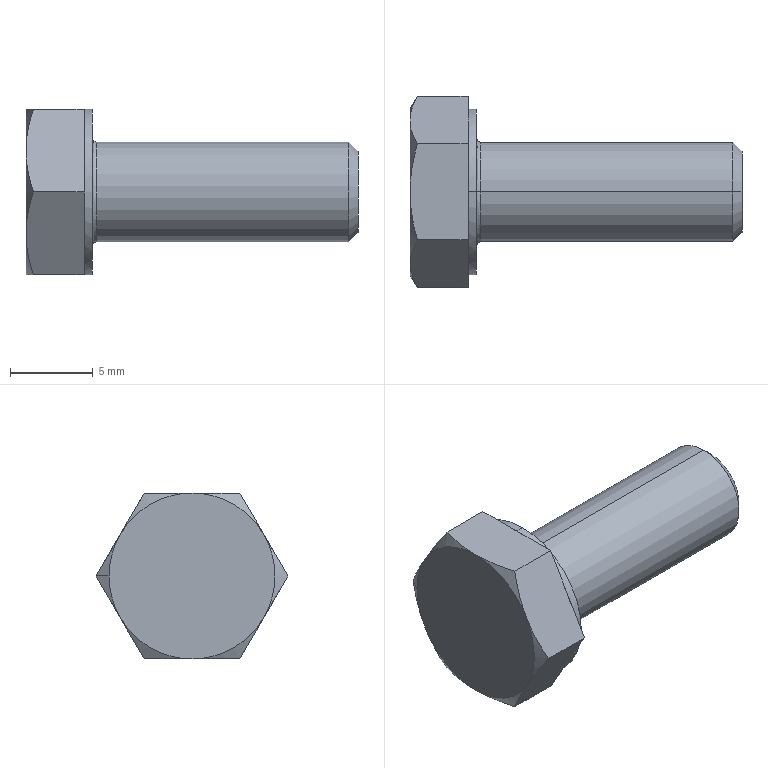Part | STEP file | Microwave Drying Flat Conveyor-hex screw gradeab_din_DIN EN 24017 - M6 x 16-N_Default | 1 solid | 30 faces | box 20 x 11.547 x 10 mm | volume 791.21 mm3 | plane 15 | cone 9 | cylinder 4 | spline 2 | commonest cylinder face diameters 6 x2 10 x2
STEP:
#1=CARTESIAN_POINT('',(4.,0.,3.25));
#2=VERTEX_POINT('',#1);
#3=CARTESIAN_POINT('',(4.,0.,-3.25));
#4=VERTEX_POINT('',#3);
#5=CARTESIAN_POINT('',(4.,0.,3.25));
#6=CARTESIAN_POINT('',(4.,0.2065,3.25));
#7=CARTESIAN_POINT('',(4.,0.511,3.221));
#8=CARTESIAN_POINT('',(4.,0.8568,3.138));
#9=CARTESIAN_POINT('',(4.,1.027,3.084));
#10=CARTESIAN_POINT('',(4.,1.1,3.058));
#11=CARTESIAN_POINT('',(4.,1.148,3.041));
#12=CARTESIAN_POINT('',(4.,1.17,3.032));
#13=CARTESIAN_POINT('',(4.,1.613,2.857));
#14=CARTESIAN_POINT('',(4.,1.981,2.615));
#15=CARTESIAN_POINT('',(4.,2.457,2.14));
#16=CARTESIAN_POINT('',(4.,2.666,1.883));
#17=CARTESIAN_POINT('',(4.,2.861,1.551));
#18=CARTESIAN_POINT('',(4.,2.945,1.376));
#19=CARTESIAN_POINT('',(4.,2.985,1.287));
#20=CARTESIAN_POINT('',(4.,3.001,1.248));
#21=CARTESIAN_POINT('',(4.,3.011,1.222));
#22=CARTESIAN_POINT('',(4.,3.017,1.208));
#23=CARTESIAN_POINT('',(4.,3.174,0.8124));
#24=CARTESIAN_POINT('',(4.,3.25,0.4129));
#25=CARTESIAN_POINT('',(4.,3.25,-0.2065));
#26=CARTESIAN_POINT('',(4.,3.222,-0.5109));
#27=CARTESIAN_POINT('',(4.,3.138,-0.8567));
#28=CARTESIAN_POINT('',(4.,3.084,-1.027));
#29=CARTESIAN_POINT('',(4.,3.058,-1.1));
#30=CARTESIAN_POINT('',(4.,3.041,-1.148));
#31=CARTESIAN_POINT('',(4.,3.032,-1.17));
#32=CARTESIAN_POINT('',(4.,2.857,-1.613));
#33=CARTESIAN_POINT('',(4.,2.615,-1.981));
#34=CARTESIAN_POINT('',(4.,2.14,-2.457));
#35=CARTESIAN_POINT('',(4.,1.883,-2.666));
#36=CARTESIAN_POINT('',(4.,1.551,-2.861));
#37=CARTESIAN_POINT('',(4.,1.376,-2.945));
#38=CARTESIAN_POINT('',(4.,1.3,-2.979));
#39=CARTESIAN_POINT('',(4.,1.248,-3.001));
#40=CARTESIAN_POINT('',(4.,1.22,-3.012));
#41=CARTESIAN_POINT('',(4.,0.8122,-3.174));
#42=CARTESIAN_POINT('',(4.,0.4135,-3.25));
#43=CARTESIAN_POINT('',(4.,0.,-3.25));
#44=B_SPLINE_CURVE_WITH_KNOTS('',3,(#5,#6,#7,#8,#9,#10,#11,#12,#13,#14,#15,#16,#17,#18,#19,#20,#21,#22,#23,#24,#25,#26,#27,#28,#29,#30,#31,#32,#33,#34,#35,#36,#37,#38,#39,#40,#41,#42,#43),.UNSPECIFIED.,.F.,.F.,(4,1,1,1,2,2,2,1,1,1,1,2,2,2,1,1,1,2,2,2,1,1,1,2,2,4),(0.,0.0625,0.09375,0.1094,0.1172,0.125,0.25,0.3125,0.3437,0.3594,0.3672,0.3711,0.375,0.5,0.5625,0.5937,0.6094,0.6172,0.625,0.75,0.8125,0.8437,0.8594,0.8672,0.875,1.),.UNSPECIFIED.);
#45=EDGE_CURVE('',#2,#4,#44,.T.);
#46=ORIENTED_EDGE('',*,*,#45,.F.);
#47=CARTESIAN_POINT('',(4.25,0.,3.));
#48=VERTEX_POINT('',#47);
#49=CARTESIAN_POINT('',(4.25,0.,3.25));
#50=DIRECTION('',(0.,-1.,0.));
#51=DIRECTION('',(0.,0.,1.));
#52=AXIS2_PLACEMENT_3D('',#49,#50,#51);
#53=CIRCLE('',#52,0.25);
#54=EDGE_CURVE('',#2,#48,#53,.T.);
#55=ORIENTED_EDGE('',*,*,#54,.T.);
#56=CARTESIAN_POINT('',(4.25,0.,-3.));
#57=VERTEX_POINT('',#56);
#58=CARTESIAN_POINT('',(4.25,0.,0.));
#59=DIRECTION('',(1.,0.,0.));
#60=DIRECTION('',(0.,0.,1.));
#61=AXIS2_PLACEMENT_3D('',#58,#59,#60);
#62=CIRCLE('',#61,3.);
#63=EDGE_CURVE('',#57,#48,#62,.T.);
#64=ORIENTED_EDGE('',*,*,#63,.F.);
#65=CARTESIAN_POINT('',(4.25,0.,-3.25));
#66=DIRECTION('',(0.,1.,0.));
#67=DIRECTION('',(0.,0.,-1.));
#68=AXIS2_PLACEMENT_3D('',#65,#66,#67);
#69=CIRCLE('',#68,0.25);
#70=EDGE_CURVE('',#4,#57,#69,.T.);
#71=ORIENTED_EDGE('',*,*,#70,.F.);
#72=EDGE_LOOP('',(#46,#55,#64,#71));
#73=FACE_OUTER_BOUND('',#72,.T.);
#74=CARTESIAN_POINT('',(4.,0.,-3.25));
#75=CARTESIAN_POINT('',(4.,6.5,-3.25));
#76=CARTESIAN_POINT('',(4.,6.5,3.25));
#77=CARTESIAN_POINT('',(4.,0.,3.25));
#78=CARTESIAN_POINT('',(4.,0.,-3.104));
#79=CARTESIAN_POINT('',(4.,6.207,-3.104));
#80=CARTESIAN_POINT('',(4.,6.207,3.104));
#81=CARTESIAN_POINT('',(4.,0.,3.104));
#82=CARTESIAN_POINT('',(4.104,0.,-3.));
#83=CARTESIAN_POINT('',(4.104,6.,-3.));
#84=CARTESIAN_POINT('',(4.104,6.,3.));
#85=CARTESIAN_POINT('',(4.104,0.,3.));
#86=CARTESIAN_POINT('',(4.25,0.,-3.));
#87=CARTESIAN_POINT('',(4.25,6.,-3.));
#88=CARTESIAN_POINT('',(4.25,6.,3.));
#89=CARTESIAN_POINT('',(4.25,0.,3.));
#90=(BOUNDED_SURFACE()B_SPLINE_SURFACE(3,3,((#74,#75,#76,#77),(#78,#79,#80,#81),(#82,#83,#84,#85),(#86,#87,#88,#89)),.UNSPECIFIED.,.F.,.F.,.T.)B_SPLINE_SURFACE_WITH_KNOTS((4,4),(4,4),(0.,1.),(0.,1.),.UNSPECIFIED.)GEOMETRIC_REPRESENTATION_ITEM()RATIONAL_B_SPLINE_SURFACE(((1.,0.3333,0.3333,1.),(0.8047,0.2682,0.2682,0.8047),(0.8047,0.2682,0.2682,0.8047),(1.,0.3333,0.3333,1.)))REPRESENTATION_ITEM('')SURFACE());
#91=ADVANCED_FACE('',(#73),#90,.F.);
#92=CARTESIAN_POINT('',(19.445,0.,3.));
#93=VERTEX_POINT('',#92);
#94=CARTESIAN_POINT('',(19.445,0.,-3.));
#95=VERTEX_POINT('',#94);
#96=CARTESIAN_POINT('',(19.445,0.,0.));
#97=DIRECTION('',(-1.,0.,0.));
#98=DIRECTION('',(0.,0.,1.));
#99=AXIS2_PLACEMENT_3D('',#96,#97,#98);
#100=CIRCLE('',#99,3.);
#101=EDGE_CURVE('',#93,#95,#100,.T.);
#102=ORIENTED_EDGE('',*,*,#101,.T.);
#103=CARTESIAN_POINT('',(0.,0.,-3.));
#104=DIRECTION('',(-1.,0.,0.));
#105=VECTOR('',#104,1000.);
#106=LINE('',#103,#105);
#107=EDGE_CURVE('',#95,#57,#106,.T.);
#108=ORIENTED_EDGE('',*,*,#107,.T.);
#109=ORIENTED_EDGE('',*,*,#63,.T.);
#110=CARTESIAN_POINT('',(0.,0.,3.));
#111=DIRECTION('',(-1.,0.,0.));
#112=VECTOR('',#111,1000.);
#113=LINE('',#110,#112);
#114=EDGE_CURVE('',#93,#48,#113,.T.);
#115=ORIENTED_EDGE('',*,*,#114,.F.);
#116=EDGE_LOOP('',(#102,#108,#109,#115));
#117=FACE_OUTER_BOUND('',#116,.T.);
#118=CARTESIAN_POINT('',(0.,0.,0.));
#119=DIRECTION('',(-1.,0.,0.));
#120=DIRECTION('',(0.,0.,1.));
#121=AXIS2_PLACEMENT_3D('',#118,#119,#120);
#122=CYLINDRICAL_SURFACE('',#121,3.);
#123=ADVANCED_FACE('',(#117),#122,.T.);
#124=CARTESIAN_POINT('',(20.,0.,2.446));
#125=VERTEX_POINT('',#124);
#126=CARTESIAN_POINT('',(20.,0.,-2.446));
#127=VERTEX_POINT('',#126);
#128=CARTESIAN_POINT('',(20.,0.,0.));
#129=DIRECTION('',(-1.,0.,0.));
#130=DIRECTION('',(0.,0.,1.));
#131=AXIS2_PLACEMENT_3D('',#128,#129,#130);
#132=CIRCLE('',#131,2.446);
#133=EDGE_CURVE('',#125,#127,#132,.T.);
#134=ORIENTED_EDGE('',*,*,#133,.T.);
#135=CARTESIAN_POINT('',(19.446,0.,-3.));
#136=DIRECTION('',(-0.7071,0.,-0.7071));
#137=VECTOR('',#136,1000.);
#138=LINE('',#135,#137);
#139=EDGE_CURVE('',#127,#95,#138,.T.);
#140=ORIENTED_EDGE('',*,*,#139,.T.);
#141=ORIENTED_EDGE('',*,*,#101,.F.);
#142=CARTESIAN_POINT('',(19.446,0.,3.));
#143=DIRECTION('',(-0.7071,0.,0.7071));
#144=VECTOR('',#143,1000.);
#145=LINE('',#142,#144);
#146=EDGE_CURVE('',#125,#93,#145,.T.);
#147=ORIENTED_EDGE('',*,*,#146,.F.);
#148=EDGE_LOOP('',(#134,#140,#141,#147));
#149=FACE_OUTER_BOUND('',#148,.T.);
#150=CARTESIAN_POINT('',(19.446,0.,0.));
#151=DIRECTION('',(-1.,0.,0.));
#152=DIRECTION('',(0.,0.,1.));
#153=AXIS2_PLACEMENT_3D('',#150,#151,#152);
#154=CONICAL_SURFACE('',#153,3.,0.7854);
#155=ADVANCED_FACE('',(#149),#154,.T.);
#156=CARTESIAN_POINT('',(4.,0.,-5.));
#157=VERTEX_POINT('',#156);
#158=CARTESIAN_POINT('',(4.,0.,5.));
#159=VERTEX_POINT('',#158);
#160=CARTESIAN_POINT('',(4.,0.,0.));
#161=DIRECTION('',(1.,0.,0.));
#162=DIRECTION('',(0.,0.,1.));
#163=AXIS2_PLACEMENT_3D('',#160,#161,#162);
#164=CIRCLE('',#163,5.);
#165=EDGE_CURVE('',#157,#159,#164,.T.);
#166=ORIENTED_EDGE('',*,*,#165,.F.);
#167=CARTESIAN_POINT('',(3.5,0.,-5.));
#168=VERTEX_POINT('',#167);
#169=CARTESIAN_POINT('',(0.,0.,-5.));
#170=DIRECTION('',(-1.,0.,0.));
#171=VECTOR('',#170,1000.);
#172=LINE('',#169,#171);
#173=EDGE_CURVE('',#157,#168,#172,.T.);
#174=ORIENTED_EDGE('',*,*,#173,.T.);
#175=CARTESIAN_POINT('',(3.5,4.33,-2.5));
#176=VERTEX_POINT('',#175);
#177=CARTESIAN_POINT('',(3.5,0.,0.));
#178=DIRECTION('',(1.,0.,0.));
#179=DIRECTION('',(0.,0.,1.));
#180=AXIS2_PLACEMENT_3D('',#177,#178,#179);
#181=CIRCLE('',#180,5.);
#182=EDGE_CURVE('',#168,#176,#181,.T.);
#183=ORIENTED_EDGE('',*,*,#182,.T.);
#184=CARTESIAN_POINT('',(3.5,4.33,2.5));
#185=VERTEX_POINT('',#184);
#186=CARTESIAN_POINT('',(3.5,0.,0.));
#187=DIRECTION('',(1.,0.,0.));
#188=DIRECTION('',(0.,0.,1.));
#189=AXIS2_PLACEMENT_3D('',#186,#187,#188);
#190=CIRCLE('',#189,5.);
#191=EDGE_CURVE('',#176,#185,#190,.T.);
#192=ORIENTED_EDGE('',*,*,#191,.T.);
#193=CARTESIAN_POINT('',(3.5,0.,5.));
#194=VERTEX_POINT('',#193);
#195=CARTESIAN_POINT('',(3.5,0.,0.));
#196=DIRECTION('',(1.,0.,0.));
#197=DIRECTION('',(0.,0.,1.));
#198=AXIS2_PLACEMENT_3D('',#195,#196,#197);
#199=CIRCLE('',#198,5.);
#200=EDGE_CURVE('',#185,#194,#199,.T.);
#201=ORIENTED_EDGE('',*,*,#200,.T.);
#202=CARTESIAN_POINT('',(0.,0.,5.));
#203=DIRECTION('',(-1.,0.,0.));
#204=VECTOR('',#203,1000.);
#205=LINE('',#202,#204);
#206=EDGE_CURVE('',#159,#194,#205,.T.);
#207=ORIENTED_EDGE('',*,*,#206,.F.);
#208=EDGE_LOOP('',(#166,#174,#183,#192,#201,#207));
#209=FACE_OUTER_BOUND('',#208,.T.);
#210=CARTESIAN_POINT('',(0.,0.,0.));
#211=DIRECTION('',(-1.,0.,0.));
#212=DIRECTION('',(0.,0.,1.));
#213=AXIS2_PLACEMENT_3D('',#210,#211,#212);
#214=CYLINDRICAL_SURFACE('',#213,5.);
#215=ADVANCED_FACE('',(#209),#214,.T.);
#216=CARTESIAN_POINT('',(0.,4.33,-2.5));
#217=VERTEX_POINT('',#216);
#218=CARTESIAN_POINT('',(0.,5.,0.));
#219=VERTEX_POINT('',#218);
#220=CARTESIAN_POINT('',(0.,0.,0.));
#221=DIRECTION('',(1.,0.,0.));
#222=DIRECTION('',(0.,1.,0.));
#223=AXIS2_PLACEMENT_3D('',#220,#221,#222);
#224=CIRCLE('',#223,5.);
#225=EDGE_CURVE('',#217,#219,#224,.T.);
#226=ORIENTED_EDGE('',*,*,#225,.T.);
#227=CARTESIAN_POINT('',(0.4466,5.774,0.));
#228=VERTEX_POINT('',#227);
#229=CARTESIAN_POINT('',(0.4493,5.778,0.));
#230=DIRECTION('',(0.5,0.866,0.));
#231=VECTOR('',#230,1000.);
#232=LINE('',#229,#231);
#233=EDGE_CURVE('',#219,#228,#232,.T.);
#234=ORIENTED_EDGE('',*,*,#233,.T.);
#235=CARTESIAN_POINT('',(0.4466,5.774,0.));
#236=CARTESIAN_POINT('',(0.1743,5.302,-0.8168));
#237=CARTESIAN_POINT('',(0.,4.823,-1.647));
#238=CARTESIAN_POINT('',(0.,4.33,-2.5));
#239=B_SPLINE_CURVE_WITH_KNOTS('',3,(#235,#236,#237,#238),.UNSPECIFIED.,.F.,.F.,(4,4),(0.,0.002921),.UNSPECIFIED.);
#240=EDGE_CURVE('',#228,#217,#239,.T.);
#241=ORIENTED_EDGE('',*,*,#240,.T.);
#242=EDGE_LOOP('',(#226,#234,#241));
#243=FACE_OUTER_BOUND('',#242,.T.);
#244=CARTESIAN_POINT('',(0.4493,0.,0.));
#245=DIRECTION('',(1.,0.,0.));
#246=DIRECTION('',(0.,1.,0.));
#247=AXIS2_PLACEMENT_3D('',#244,#245,#246);
#248=CONICAL_SURFACE('',#247,5.778,1.047);
#249=ADVANCED_FACE('',(#243),#248,.T.);
#250=ORIENTED_EDGE('',*,*,#107,.F.);
#251=CARTESIAN_POINT('',(19.445,0.,0.));
#252=DIRECTION('',(-1.,0.,0.));
#253=DIRECTION('',(0.,0.,1.));
#254=AXIS2_PLACEMENT_3D('',#251,#252,#253);
#255=CIRCLE('',#254,3.);
#256=EDGE_CURVE('',#95,#93,#255,.T.);
#257=ORIENTED_EDGE('',*,*,#256,.T.);
#258=ORIENTED_EDGE('',*,*,#114,.T.);
#259=CARTESIAN_POINT('',(4.25,0.,0.));
#260=DIRECTION('',(1.,0.,0.));
#261=DIRECTION('',(0.,0.,1.));
#262=AXIS2_PLACEMENT_3D('',#259,#260,#261);
#263=CIRCLE('',#262,3.);
#264=EDGE_CURVE('',#48,#57,#263,.T.);
#265=ORIENTED_EDGE('',*,*,#264,.T.);
#266=EDGE_LOOP('',(#250,#257,#258,#265));
#267=FACE_OUTER_BOUND('',#266,.T.);
#268=CARTESIAN_POINT('',(0.,0.,0.));
#269=DIRECTION('',(-1.,0.,0.));
#270=DIRECTION('',(0.,0.,1.));
#271=AXIS2_PLACEMENT_3D('',#268,#269,#270);
#272=CYLINDRICAL_SURFACE('',#271,3.);
#273=ADVANCED_FACE('',(#267),#272,.T.);
#274=ORIENTED_EDGE('',*,*,#54,.F.);
#275=CARTESIAN_POINT('',(4.,0.,-3.25));
#276=CARTESIAN_POINT('',(4.,-0.2065,-3.25));
#277=CARTESIAN_POINT('',(4.,-0.511,-3.221));
#278=CARTESIAN_POINT('',(4.,-0.8568,-3.138));
#279=CARTESIAN_POINT('',(4.,-1.027,-3.084));
#280=CARTESIAN_POINT('',(4.,-1.1,-3.058));
#281=CARTESIAN_POINT('',(4.,-1.148,-3.041));
#282=CARTESIAN_POINT('',(4.,-1.17,-3.032));
#283=CARTESIAN_POINT('',(4.,-1.613,-2.857));
#284=CARTESIAN_POINT('',(4.,-1.981,-2.615));
#285=CARTESIAN_POINT('',(4.,-2.457,-2.14));
#286=CARTESIAN_POINT('',(4.,-2.666,-1.883));
#287=CARTESIAN_POINT('',(4.,-2.861,-1.551));
#288=CARTESIAN_POINT('',(4.,-2.945,-1.376));
#289=CARTESIAN_POINT('',(4.,-2.985,-1.287));
#290=CARTESIAN_POINT('',(4.,-3.001,-1.248));
#291=CARTESIAN_POINT('',(4.,-3.011,-1.222));
#292=CARTESIAN_POINT('',(4.,-3.017,-1.208));
#293=CARTESIAN_POINT('',(4.,-3.174,-0.8124));
#294=CARTESIAN_POINT('',(4.,-3.25,-0.4129));
#295=CARTESIAN_POINT('',(4.,-3.25,0.2065));
#296=CARTESIAN_POINT('',(4.,-3.222,0.5109));
#297=CARTESIAN_POINT('',(4.,-3.138,0.8567));
#298=CARTESIAN_POINT('',(4.,-3.084,1.027));
#299=CARTESIAN_POINT('',(4.,-3.058,1.1));
#300=CARTESIAN_POINT('',(4.,-3.041,1.148));
#301=CARTESIAN_POINT('',(4.,-3.032,1.17));
#302=CARTESIAN_POINT('',(4.,-2.857,1.613));
#303=CARTESIAN_POINT('',(4.,-2.615,1.981));
#304=CARTESIAN_POINT('',(4.,-2.14,2.457));
#305=CARTESIAN_POINT('',(4.,-1.883,2.666));
#306=CARTESIAN_POINT('',(4.,-1.551,2.861));
#307=CARTESIAN_POINT('',(4.,-1.376,2.945));
#308=CARTESIAN_POINT('',(4.,-1.3,2.979));
#309=CARTESIAN_POINT('',(4.,-1.248,3.001));
#310=CARTESIAN_POINT('',(4.,-1.22,3.012));
#311=CARTESIAN_POINT('',(4.,-0.8122,3.174));
#312=CARTESIAN_POINT('',(4.,-0.4135,3.25));
#313=CARTESIAN_POINT('',(4.,0.,3.25));
#314=B_SPLINE_CURVE_WITH_KNOTS('',3,(#275,#276,#277,#278,#279,#280,#281,#282,#283,#284,#285,#286,#287,#288,#289,#290,#291,#292,#293,#294,#295,#296,#297,#298,#299,#300,#301,#302,#303,#304,#305,#306,#307,#308,#309,#310,#311,#312,#313),.UNSPECIFIED.,.F.,.F.,(4,1,1,1,2,2,2,1,1,1,1,2,2,2,1,1,1,2,2,2,1,1,1,2,2,4),(0.,0.0625,0.09375,0.1094,0.1172,0.125,0.25,0.3125,0.3437,0.3594,0.3672,0.3711,0.375,0.5,0.5625,0.5937,0.6094,0.6172,0.625,0.75,0.8125,0.8437,0.8594,0.8672,0.875,1.),.UNSPECIFIED.);
#315=EDGE_CURVE('',#4,#2,#314,.T.);
#316=ORIENTED_EDGE('',*,*,#315,.F.);
#317=ORIENTED_EDGE('',*,*,#70,.T.);
#318=ORIENTED_EDGE('',*,*,#264,.F.);
#319=EDGE_LOOP('',(#274,#316,#317,#318));
#320=FACE_OUTER_BOUND('',#319,.T.);
#321=CARTESIAN_POINT('',(4.,0.,3.25));
#322=CARTESIAN_POINT('',(4.,-6.5,3.25));
#323=CARTESIAN_POINT('',(4.,-6.5,-3.25));
#324=CARTESIAN_POINT('',(4.,0.,-3.25));
#325=CARTESIAN_POINT('',(4.,0.,3.104));
#326=CARTESIAN_POINT('',(4.,-6.207,3.104));
#327=CARTESIAN_POINT('',(4.,-6.207,-3.104));
#328=CARTESIAN_POINT('',(4.,0.,-3.104));
#329=CARTESIAN_POINT('',(4.104,0.,3.));
#330=CARTESIAN_POINT('',(4.104,-6.,3.));
#331=CARTESIAN_POINT('',(4.104,-6.,-3.));
#332=CARTESIAN_POINT('',(4.104,0.,-3.));
#333=CARTESIAN_POINT('',(4.25,0.,3.));
#334=CARTESIAN_POINT('',(4.25,-6.,3.));
#335=CARTESIAN_POINT('',(4.25,-6.,-3.));
#336=CARTESIAN_POINT('',(4.25,0.,-3.));
#337=(BOUNDED_SURFACE()B_SPLINE_SURFACE(3,3,((#321,#322,#323,#324),(#325,#326,#327,#328),(#329,#330,#331,#332),(#333,#334,#335,#336)),.UNSPECIFIED.,.F.,.F.,.T.)B_SPLINE_SURFACE_WITH_KNOTS((4,4),(4,4),(0.,1.),(0.,1.),.UNSPECIFIED.)GEOMETRIC_REPRESENTATION_ITEM()RATIONAL_B_SPLINE_SURFACE(((1.,0.3333,0.3333,1.),(0.8047,0.2682,0.2682,0.8047),(0.8047,0.2682,0.2682,0.8047),(1.,0.3333,0.3333,1.)))REPRESENTATION_ITEM('')SURFACE());
#338=ADVANCED_FACE('',(#320),#337,.F.);
#339=ORIENTED_EDGE('',*,*,#139,.F.);
#340=CARTESIAN_POINT('',(20.,0.,0.));
#341=DIRECTION('',(-1.,0.,0.));
#342=DIRECTION('',(0.,0.,1.));
#343=AXIS2_PLACEMENT_3D('',#340,#341,#342);
#344=CIRCLE('',#343,2.446);
#345=EDGE_CURVE('',#127,#125,#344,.T.);
#346=ORIENTED_EDGE('',*,*,#345,.T.);
#347=ORIENTED_EDGE('',*,*,#146,.T.);
#348=ORIENTED_EDGE('',*,*,#256,.F.);
#349=EDGE_LOOP('',(#339,#346,#347,#348));
#350=FACE_OUTER_BOUND('',#349,.T.);
#351=CARTESIAN_POINT('',(19.446,0.,0.));
#352=DIRECTION('',(-1.,0.,0.));
#353=DIRECTION('',(0.,0.,1.));
#354=AXIS2_PLACEMENT_3D('',#351,#352,#353);
#355=CONICAL_SURFACE('',#354,3.,0.7854);
#356=ADVANCED_FACE('',(#350),#355,.T.);
#357=CARTESIAN_POINT('',(4.,0.,0.));
#358=DIRECTION('',(1.,0.,0.));
#359=DIRECTION('',(0.,0.,1.));
#360=AXIS2_PLACEMENT_3D('',#357,#358,#359);
#361=CIRCLE('',#360,5.);
#362=EDGE_CURVE('',#159,#157,#361,.T.);
#363=ORIENTED_EDGE('',*,*,#362,.T.);
#364=ORIENTED_EDGE('',*,*,#165,.T.);
#365=EDGE_LOOP('',(#363,#364));
#366=FACE_OUTER_BOUND('',#365,.T.);
#367=ORIENTED_EDGE('',*,*,#315,.T.);
#368=ORIENTED_EDGE('',*,*,#45,.T.);
#369=EDGE_LOOP('',(#367,#368));
#370=FACE_BOUND('',#369,.T.);
#371=CARTESIAN_POINT('',(4.,5.774,0.));
#372=DIRECTION('',(1.,0.,0.));
#373=DIRECTION('',(0.,0.,-1.));
#374=AXIS2_PLACEMENT_3D('',#371,#372,#373);
#375=PLANE('',#374);
#376=ADVANCED_FACE('',(#366,#370),#375,.T.);
#377=ORIENTED_EDGE('',*,*,#133,.F.);
#378=ORIENTED_EDGE('',*,*,#345,.F.);
#379=EDGE_LOOP('',(#377,#378));
#380=FACE_OUTER_BOUND('',#379,.T.);
#381=CARTESIAN_POINT('',(20.,0.,0.));
#382=DIRECTION('',(-1.,0.,0.));
#383=DIRECTION('',(0.,0.,1.));
#384=AXIS2_PLACEMENT_3D('',#381,#382,#383);
#385=PLANE('',#384);
#386=ADVANCED_FACE('',(#380),#385,.F.);
#387=ORIENTED_EDGE('',*,*,#173,.F.);
#388=ORIENTED_EDGE('',*,*,#362,.F.);
#389=ORIENTED_EDGE('',*,*,#206,.T.);
#390=CARTESIAN_POINT('',(3.5,-4.33,2.5));
#391=VERTEX_POINT('',#390);
#392=CARTESIAN_POINT('',(3.5,0.,0.));
#393=DIRECTION('',(1.,0.,0.));
#394=DIRECTION('',(0.,0.,1.));
#395=AXIS2_PLACEMENT_3D('',#392,#393,#394);
#396=CIRCLE('',#395,5.);
#397=EDGE_CURVE('',#194,#391,#396,.T.);
#398=ORIENTED_EDGE('',*,*,#397,.T.);
#399=CARTESIAN_POINT('',(3.5,-4.33,-2.5));
#400=VERTEX_POINT('',#399);
#401=CARTESIAN_POINT('',(3.5,0.,0.));
#402=DIRECTION('',(1.,0.,0.));
#403=DIRECTION('',(0.,0.,1.));
#404=AXIS2_PLACEMENT_3D('',#401,#402,#403);
#405=CIRCLE('',#404,5.);
#406=EDGE_CURVE('',#391,#400,#405,.T.);
#407=ORIENTED_EDGE('',*,*,#406,.T.);
#408=CARTESIAN_POINT('',(3.5,0.,0.));
#409=DIRECTION('',(1.,0.,0.));
#410=DIRECTION('',(0.,0.,1.));
#411=AXIS2_PLACEMENT_3D('',#408,#409,#410);
#412=CIRCLE('',#411,5.);
#413=EDGE_CURVE('',#400,#168,#412,.T.);
#414=ORIENTED_EDGE('',*,*,#413,.T.);
#415=EDGE_LOOP('',(#387,#388,#389,#398,#407,#414));
#416=FACE_OUTER_BOUND('',#415,.T.);
#417=CARTESIAN_POINT('',(0.,0.,0.));
#418=DIRECTION('',(-1.,0.,0.));
#419=DIRECTION('',(0.,0.,1.));
#420=AXIS2_PLACEMENT_3D('',#417,#418,#419);
#421=CYLINDRICAL_SURFACE('',#420,5.);
#422=ADVANCED_FACE('',(#416),#421,.T.);
#423=CARTESIAN_POINT('',(3.5,2.887,5.));
#424=VERTEX_POINT('',#423);
#425=CARTESIAN_POINT('',(3.5,5.,5.));
#426=DIRECTION('',(0.,-1.,0.));
#427=VECTOR('',#426,1000.);
#428=LINE('',#425,#427);
#429=EDGE_CURVE('',#424,#194,#428,.T.);
#430=ORIENTED_EDGE('',*,*,#429,.T.);
#431=ORIENTED_EDGE('',*,*,#200,.F.);
#432=CARTESIAN_POINT('',(3.5,4.33,2.5));
#433=DIRECTION('',(0.,-0.5,0.866));
#434=VECTOR('',#433,1000.);
#435=LINE('',#432,#434);
#436=EDGE_CURVE('',#185,#424,#435,.T.);
#437=ORIENTED_EDGE('',*,*,#436,.T.);
#438=EDGE_LOOP('',(#430,#431,#437));
#439=FACE_OUTER_BOUND('',#438,.T.);
#440=CARTESIAN_POINT('',(3.5,5.,0.));
#441=DIRECTION('',(1.,0.,0.));
#442=DIRECTION('',(0.,0.,-1.));
#443=AXIS2_PLACEMENT_3D('',#440,#441,#442);
#444=PLANE('',#443);
#445=ADVANCED_FACE('',(#439),#444,.T.);
#446=CARTESIAN_POINT('',(3.5,5.774,0.));
#447=VERTEX_POINT('',#446);
#448=CARTESIAN_POINT('',(3.5,5.774,0.));
#449=DIRECTION('',(0.,-0.5,0.866));
#450=VECTOR('',#449,1000.);
#451=LINE('',#448,#450);
#452=EDGE_CURVE('',#447,#185,#451,.T.);
#453=ORIENTED_EDGE('',*,*,#452,.T.);
#454=ORIENTED_EDGE('',*,*,#191,.F.);
#455=CARTESIAN_POINT('',(3.5,4.33,-2.5));
#456=DIRECTION('',(0.,0.5,0.866));
#457=VECTOR('',#456,1000.);
#458=LINE('',#455,#457);
#459=EDGE_CURVE('',#176,#447,#458,.T.);
#460=ORIENTED_EDGE('',*,*,#459,.T.);
#461=EDGE_LOOP('',(#453,#454,#460));
#462=FACE_OUTER_BOUND('',#461,.T.);
#463=CARTESIAN_POINT('',(3.5,5.,0.));
#464=DIRECTION('',(1.,0.,0.));
#465=DIRECTION('',(0.,0.,-1.));
#466=AXIS2_PLACEMENT_3D('',#463,#464,#465);
#467=PLANE('',#466);
#468=ADVANCED_FACE('',(#462),#467,.T.);
#469=ORIENTED_EDGE('',*,*,#182,.F.);
#470=CARTESIAN_POINT('',(3.5,2.887,-5.));
#471=VERTEX_POINT('',#470);
#472=CARTESIAN_POINT('',(3.5,5.,-5.));
#473=DIRECTION('',(0.,1.,0.));
#474=VECTOR('',#473,1000.);
#475=LINE('',#472,#474);
#476=EDGE_CURVE('',#168,#471,#475,.T.);
#477=ORIENTED_EDGE('',*,*,#476,.T.);
#478=CARTESIAN_POINT('',(3.5,2.887,-5.));
#479=DIRECTION('',(0.,0.5,0.866));
#480=VECTOR('',#479,1000.);
#481=LINE('',#478,#480);
#482=EDGE_CURVE('',#471,#176,#481,.T.);
#483=ORIENTED_EDGE('',*,*,#482,.T.);
#484=EDGE_LOOP('',(#469,#477,#483));
#485=FACE_OUTER_BOUND('',#484,.T.);
#486=CARTESIAN_POINT('',(3.5,5.,0.));
#487=DIRECTION('',(1.,0.,0.));
#488=DIRECTION('',(0.,0.,-1.));
#489=AXIS2_PLACEMENT_3D('',#486,#487,#488);
#490=PLANE('',#489);
#491=ADVANCED_FACE('',(#485),#490,.T.);
#492=CARTESIAN_POINT('',(3.5,-2.887,-5.));
#493=VERTEX_POINT('',#492);
#494=CARTESIAN_POINT('',(3.5,5.,-5.));
#495=DIRECTION('',(0.,1.,0.));
#496=VECTOR('',#495,1000.);
#497=LINE('',#494,#496);
#498=EDGE_CURVE('',#493,#168,#497,.T.);
#499=ORIENTED_EDGE('',*,*,#498,.T.);
#500=ORIENTED_EDGE('',*,*,#413,.F.);
#501=CARTESIAN_POINT('',(3.5,-4.33,-2.5));
#502=DIRECTION('',(0.,0.5,-0.866));
#503=VECTOR('',#502,1000.);
#504=LINE('',#501,#503);
#505=EDGE_CURVE('',#400,#493,#504,.T.);
#506=ORIENTED_EDGE('',*,*,#505,.T.);
#507=EDGE_LOOP('',(#499,#500,#506));
#508=FACE_OUTER_BOUND('',#507,.T.);
#509=CARTESIAN_POINT('',(3.5,5.,0.));
#510=DIRECTION('',(1.,0.,0.));
#511=DIRECTION('',(0.,0.,-1.));
#512=AXIS2_PLACEMENT_3D('',#509,#510,#511);
#513=PLANE('',#512);
#514=ADVANCED_FACE('',(#508),#513,.T.);
#515=CARTESIAN_POINT('',(3.5,-5.774,0.));
#516=VERTEX_POINT('',#515);
#517=CARTESIAN_POINT('',(3.5,-5.774,0.));
#518=DIRECTION('',(0.,0.5,-0.866));
#519=VECTOR('',#518,1000.);
#520=LINE('',#517,#519);
#521=EDGE_CURVE('',#516,#400,#520,.T.);
#522=ORIENTED_EDGE('',*,*,#521,.T.);
#523=ORIENTED_EDGE('',*,*,#406,.F.);
#524=CARTESIAN_POINT('',(3.5,-4.33,2.5));
#525=DIRECTION('',(0.,-0.5,-0.866));
#526=VECTOR('',#525,1000.);
#527=LINE('',#524,#526);
#528=EDGE_CURVE('',#391,#516,#527,.T.);
#529=ORIENTED_EDGE('',*,*,#528,.T.);
#530=EDGE_LOOP('',(#522,#523,#529));
#531=FACE_OUTER_BOUND('',#530,.T.);
#532=CARTESIAN_POINT('',(3.5,5.,0.));
#533=DIRECTION('',(1.,0.,0.));
#534=DIRECTION('',(0.,0.,-1.));
#535=AXIS2_PLACEMENT_3D('',#532,#533,#534);
#536=PLANE('',#535);
#537=ADVANCED_FACE('',(#531),#536,.T.);
#538=CARTESIAN_POINT('',(3.5,-2.887,5.));
#539=VERTEX_POINT('',#538);
#540=CARTESIAN_POINT('',(3.5,-2.887,5.));
#541=DIRECTION('',(0.,-0.5,-0.866));
#542=VECTOR('',#541,1000.);
#543=LINE('',#540,#542);
#544=EDGE_CURVE('',#539,#391,#543,.T.);
#545=ORIENTED_EDGE('',*,*,#544,.T.);
#546=ORIENTED_EDGE('',*,*,#397,.F.);
#547=CARTESIAN_POINT('',(3.5,5.,5.));
#548=DIRECTION('',(0.,-1.,0.));
#549=VECTOR('',#548,1000.);
#550=LINE('',#547,#549);
#551=EDGE_CURVE('',#194,#539,#550,.T.);
#552=ORIENTED_EDGE('',*,*,#551,.T.);
#553=EDGE_LOOP('',(#545,#546,#552));
#554=FACE_OUTER_BOUND('',#553,.T.);
#555=CARTESIAN_POINT('',(3.5,5.,0.));
#556=DIRECTION('',(1.,0.,0.));
#557=DIRECTION('',(0.,0.,-1.));
#558=AXIS2_PLACEMENT_3D('',#555,#556,#557);
#559=PLANE('',#558);
#560=ADVANCED_FACE('',(#554),#559,.T.);
#561=CARTESIAN_POINT('',(0.4466,2.887,5.));
#562=VERTEX_POINT('',#561);
#563=CARTESIAN_POINT('',(4.,2.887,5.));
#564=DIRECTION('',(1.,0.,0.));
#565=VECTOR('',#564,1000.);
#566=LINE('',#563,#565);
#567=EDGE_CURVE('',#562,#424,#566,.T.);
#568=ORIENTED_EDGE('',*,*,#567,.F.);
#569=CARTESIAN_POINT('',(0.,0.,5.));
#570=VERTEX_POINT('',#569);
#571=CARTESIAN_POINT('',(0.,0.,5.));
#572=CARTESIAN_POINT('',(0.,0.9853,5.));
#573=CARTESIAN_POINT('',(0.1743,1.944,5.));
#574=CARTESIAN_POINT('',(0.4466,2.887,5.));
#575=B_SPLINE_CURVE_WITH_KNOTS('',3,(#571,#572,#573,#574),.UNSPECIFIED.,.F.,.F.,(4,4),(0.,0.002921),.UNSPECIFIED.);
#576=EDGE_CURVE('',#570,#562,#575,.T.);
#577=ORIENTED_EDGE('',*,*,#576,.F.);
#578=CARTESIAN_POINT('',(0.4466,-2.887,5.));
#579=VERTEX_POINT('',#578);
#580=CARTESIAN_POINT('',(0.4466,-2.887,5.));
#581=CARTESIAN_POINT('',(0.1743,-1.944,5.));
#582=CARTESIAN_POINT('',(0.,-0.9853,5.));
#583=CARTESIAN_POINT('',(0.,0.,5.));
#584=B_SPLINE_CURVE_WITH_KNOTS('',3,(#580,#581,#582,#583),.UNSPECIFIED.,.F.,.F.,(4,4),(0.,0.002921),.UNSPECIFIED.);
#585=EDGE_CURVE('',#579,#570,#584,.T.);
#586=ORIENTED_EDGE('',*,*,#585,.F.);
#587=CARTESIAN_POINT('',(4.,-2.887,5.));
#588=DIRECTION('',(-1.,0.,0.));
#589=VECTOR('',#588,1000.);
#590=LINE('',#587,#589);
#591=EDGE_CURVE('',#539,#579,#590,.T.);
#592=ORIENTED_EDGE('',*,*,#591,.F.);
#593=ORIENTED_EDGE('',*,*,#551,.F.);
#594=ORIENTED_EDGE('',*,*,#429,.F.);
#595=EDGE_LOOP('',(#568,#577,#586,#592,#593,#594));
#596=FACE_OUTER_BOUND('',#595,.T.);
#597=CARTESIAN_POINT('',(4.,2.887,5.));
#598=DIRECTION('',(0.,0.,-1.));
#599=DIRECTION('',(0.,1.,0.));
#600=AXIS2_PLACEMENT_3D('',#597,#598,#599);
#601=PLANE('',#600);
#602=ADVANCED_FACE('',(#596),#601,.F.);
#603=CARTESIAN_POINT('',(4.,5.774,0.));
#604=DIRECTION('',(1.,0.,0.));
#605=VECTOR('',#604,1000.);
#606=LINE('',#603,#605);
#607=EDGE_CURVE('',#228,#447,#606,.T.);
#608=ORIENTED_EDGE('',*,*,#607,.F.);
#609=CARTESIAN_POINT('',(0.,4.33,2.5));
#610=VERTEX_POINT('',#609);
#611=CARTESIAN_POINT('',(0.,4.33,2.5));
#612=CARTESIAN_POINT('',(0.,4.823,1.647));
#613=CARTESIAN_POINT('',(0.1743,5.302,0.8168));
#614=CARTESIAN_POINT('',(0.4466,5.774,0.));
#615=B_SPLINE_CURVE_WITH_KNOTS('',3,(#611,#612,#613,#614),.UNSPECIFIED.,.F.,.F.,(4,4),(0.,0.002921),.UNSPECIFIED.);
#616=EDGE_CURVE('',#610,#228,#615,.T.);
#617=ORIENTED_EDGE('',*,*,#616,.F.);
#618=CARTESIAN_POINT('',(0.4466,2.887,5.));
#619=CARTESIAN_POINT('',(0.1743,3.358,4.183));
#620=CARTESIAN_POINT('',(0.,3.837,3.353));
#621=CARTESIAN_POINT('',(0.,4.33,2.5));
#622=B_SPLINE_CURVE_WITH_KNOTS('',3,(#618,#619,#620,#621),.UNSPECIFIED.,.F.,.F.,(4,4),(0.,0.002921),.UNSPECIFIED.);
#623=EDGE_CURVE('',#562,#610,#622,.T.);
#624=ORIENTED_EDGE('',*,*,#623,.F.);
#625=ORIENTED_EDGE('',*,*,#567,.T.);
#626=ORIENTED_EDGE('',*,*,#436,.F.);
#627=ORIENTED_EDGE('',*,*,#452,.F.);
#628=EDGE_LOOP('',(#608,#617,#624,#625,#626,#627));
#629=FACE_OUTER_BOUND('',#628,.T.);
#630=CARTESIAN_POINT('',(4.,5.774,0.));
#631=DIRECTION('',(0.,-0.866,-0.5));
#632=DIRECTION('',(0.,0.5,-0.866));
#633=AXIS2_PLACEMENT_3D('',#630,#631,#632);
#634=PLANE('',#633);
#635=ADVANCED_FACE('',(#629),#634,.F.);
#636=CARTESIAN_POINT('',(0.4466,2.887,-5.));
#637=VERTEX_POINT('',#636);
#638=CARTESIAN_POINT('',(4.,2.887,-5.));
#639=DIRECTION('',(1.,0.,0.));
#640=VECTOR('',#639,1000.);
#641=LINE('',#638,#640);
#642=EDGE_CURVE('',#637,#471,#641,.T.);
#643=ORIENTED_EDGE('',*,*,#642,.F.);
#644=CARTESIAN_POINT('',(0.,4.33,-2.5));
#645=CARTESIAN_POINT('',(0.,3.837,-3.353));
#646=CARTESIAN_POINT('',(0.1743,3.358,-4.183));
#647=CARTESIAN_POINT('',(0.4466,2.887,-5.));
#648=B_SPLINE_CURVE_WITH_KNOTS('',3,(#644,#645,#646,#647),.UNSPECIFIED.,.F.,.F.,(4,4),(0.,0.002921),.UNSPECIFIED.);
#649=EDGE_CURVE('',#217,#637,#648,.T.);
#650=ORIENTED_EDGE('',*,*,#649,.F.);
#651=ORIENTED_EDGE('',*,*,#240,.F.);
#652=ORIENTED_EDGE('',*,*,#607,.T.);
#653=ORIENTED_EDGE('',*,*,#459,.F.);
#654=ORIENTED_EDGE('',*,*,#482,.F.);
#655=EDGE_LOOP('',(#643,#650,#651,#652,#653,#654));
#656=FACE_OUTER_BOUND('',#655,.T.);
#657=CARTESIAN_POINT('',(4.,2.887,-5.));
#658=DIRECTION('',(0.,-0.866,0.5));
#659=DIRECTION('',(0.,-0.5,-0.866));
#660=AXIS2_PLACEMENT_3D('',#657,#658,#659);
#661=PLANE('',#660);
#662=ADVANCED_FACE('',(#656),#661,.F.);
#663=CARTESIAN_POINT('',(0.4466,-2.887,-5.));
#664=VERTEX_POINT('',#663);
#665=CARTESIAN_POINT('',(4.,-2.887,-5.));
#666=DIRECTION('',(1.,0.,0.));
#667=VECTOR('',#666,1000.);
#668=LINE('',#665,#667);
#669=EDGE_CURVE('',#664,#493,#668,.T.);
#670=ORIENTED_EDGE('',*,*,#669,.F.);
#671=CARTESIAN_POINT('',(0.,0.,-5.));
#672=VERTEX_POINT('',#671);
#673=CARTESIAN_POINT('',(0.,0.,-5.));
#674=CARTESIAN_POINT('',(0.,-0.9853,-5.));
#675=CARTESIAN_POINT('',(0.1743,-1.944,-5.));
#676=CARTESIAN_POINT('',(0.4466,-2.887,-5.));
#677=B_SPLINE_CURVE_WITH_KNOTS('',3,(#673,#674,#675,#676),.UNSPECIFIED.,.F.,.F.,(4,4),(0.,0.002921),.UNSPECIFIED.);
#678=EDGE_CURVE('',#672,#664,#677,.T.);
#679=ORIENTED_EDGE('',*,*,#678,.F.);
#680=CARTESIAN_POINT('',(0.4466,2.887,-5.));
#681=CARTESIAN_POINT('',(0.1743,1.944,-5.));
#682=CARTESIAN_POINT('',(0.,0.9853,-5.));
#683=CARTESIAN_POINT('',(0.,0.,-5.));
#684=B_SPLINE_CURVE_WITH_KNOTS('',3,(#680,#681,#682,#683),.UNSPECIFIED.,.F.,.F.,(4,4),(0.,0.002921),.UNSPECIFIED.);
#685=EDGE_CURVE('',#637,#672,#684,.T.);
#686=ORIENTED_EDGE('',*,*,#685,.F.);
#687=ORIENTED_EDGE('',*,*,#642,.T.);
#688=ORIENTED_EDGE('',*,*,#476,.F.);
#689=ORIENTED_EDGE('',*,*,#498,.F.);
#690=EDGE_LOOP('',(#670,#679,#686,#687,#688,#689));
#691=FACE_OUTER_BOUND('',#690,.T.);
#692=CARTESIAN_POINT('',(4.,2.887,-5.));
#693=DIRECTION('',(0.,0.,1.));
#694=DIRECTION('',(0.,-1.,0.));
#695=AXIS2_PLACEMENT_3D('',#692,#693,#694);
#696=PLANE('',#695);
#697=ADVANCED_FACE('',(#691),#696,.F.);
#698=CARTESIAN_POINT('',(0.4466,-5.774,0.));
#699=VERTEX_POINT('',#698);
#700=CARTESIAN_POINT('',(4.,-5.774,0.));
#701=DIRECTION('',(1.,0.,0.));
#702=VECTOR('',#701,1000.);
#703=LINE('',#700,#702);
#704=EDGE_CURVE('',#699,#516,#703,.T.);
#705=ORIENTED_EDGE('',*,*,#704,.F.);
#706=CARTESIAN_POINT('',(0.,-4.33,-2.5));
#707=VERTEX_POINT('',#706);
#708=CARTESIAN_POINT('',(0.,-4.33,-2.5));
#709=CARTESIAN_POINT('',(0.,-4.823,-1.647));
#710=CARTESIAN_POINT('',(0.1743,-5.302,-0.8168));
#711=CARTESIAN_POINT('',(0.4466,-5.774,0.));
#712=B_SPLINE_CURVE_WITH_KNOTS('',3,(#708,#709,#710,#711),.UNSPECIFIED.,.F.,.F.,(4,4),(0.,0.002921),.UNSPECIFIED.);
#713=EDGE_CURVE('',#707,#699,#712,.T.);
#714=ORIENTED_EDGE('',*,*,#713,.F.);
#715=CARTESIAN_POINT('',(0.4466,-2.887,-5.));
#716=CARTESIAN_POINT('',(0.1743,-3.358,-4.183));
#717=CARTESIAN_POINT('',(0.,-3.837,-3.353));
#718=CARTESIAN_POINT('',(0.,-4.33,-2.5));
#719=B_SPLINE_CURVE_WITH_KNOTS('',3,(#715,#716,#717,#718),.UNSPECIFIED.,.F.,.F.,(4,4),(0.,0.002921),.UNSPECIFIED.);
#720=EDGE_CURVE('',#664,#707,#719,.T.);
#721=ORIENTED_EDGE('',*,*,#720,.F.);
#722=ORIENTED_EDGE('',*,*,#669,.T.);
#723=ORIENTED_EDGE('',*,*,#505,.F.);
#724=ORIENTED_EDGE('',*,*,#521,.F.);
#725=EDGE_LOOP('',(#705,#714,#721,#722,#723,#724));
#726=FACE_OUTER_BOUND('',#725,.T.);
#727=CARTESIAN_POINT('',(4.,-2.887,-5.));
#728=DIRECTION('',(0.,0.866,0.5));
#729=DIRECTION('',(0.,-0.5,0.866));
#730=AXIS2_PLACEMENT_3D('',#727,#728,#729);
#731=PLANE('',#730);
#732=ADVANCED_FACE('',(#726),#731,.F.);
#733=ORIENTED_EDGE('',*,*,#591,.T.);
#734=CARTESIAN_POINT('',(0.,-4.33,2.5));
#735=VERTEX_POINT('',#734);
#736=CARTESIAN_POINT('',(0.,-4.33,2.5));
#737=CARTESIAN_POINT('',(0.,-3.837,3.353));
#738=CARTESIAN_POINT('',(0.1743,-3.358,4.183));
#739=CARTESIAN_POINT('',(0.4466,-2.887,5.));
#740=B_SPLINE_CURVE_WITH_KNOTS('',3,(#736,#737,#738,#739),.UNSPECIFIED.,.F.,.F.,(4,4),(0.,0.002921),.UNSPECIFIED.);
#741=EDGE_CURVE('',#735,#579,#740,.T.);
#742=ORIENTED_EDGE('',*,*,#741,.F.);
#743=CARTESIAN_POINT('',(0.4466,-5.774,0.));
#744=CARTESIAN_POINT('',(0.1743,-5.302,0.8168));
#745=CARTESIAN_POINT('',(0.,-4.823,1.647));
#746=CARTESIAN_POINT('',(0.,-4.33,2.5));
#747=B_SPLINE_CURVE_WITH_KNOTS('',3,(#743,#744,#745,#746),.UNSPECIFIED.,.F.,.F.,(4,4),(0.,0.002921),.UNSPECIFIED.);
#748=EDGE_CURVE('',#699,#735,#747,.T.);
#749=ORIENTED_EDGE('',*,*,#748,.F.);
#750=ORIENTED_EDGE('',*,*,#704,.T.);
#751=ORIENTED_EDGE('',*,*,#528,.F.);
#752=ORIENTED_EDGE('',*,*,#544,.F.);
#753=EDGE_LOOP('',(#733,#742,#749,#750,#751,#752));
#754=FACE_OUTER_BOUND('',#753,.T.);
#755=CARTESIAN_POINT('',(4.,-5.774,0.));
#756=DIRECTION('',(0.,0.866,-0.5));
#757=DIRECTION('',(0.,0.5,0.866));
#758=AXIS2_PLACEMENT_3D('',#755,#756,#757);
#759=PLANE('',#758);
#760=ADVANCED_FACE('',(#754),#759,.F.);
#761=ORIENTED_EDGE('',*,*,#623,.T.);
#762=CARTESIAN_POINT('',(0.,0.,0.));
#763=DIRECTION('',(1.,0.,0.));
#764=DIRECTION('',(0.,1.,0.));
#765=AXIS2_PLACEMENT_3D('',#762,#763,#764);
#766=CIRCLE('',#765,5.);
#767=EDGE_CURVE('',#610,#570,#766,.T.);
#768=ORIENTED_EDGE('',*,*,#767,.T.);
#769=ORIENTED_EDGE('',*,*,#576,.T.);
#770=EDGE_LOOP('',(#761,#768,#769));
#771=FACE_OUTER_BOUND('',#770,.T.);
#772=CARTESIAN_POINT('',(0.4493,0.,0.));
#773=DIRECTION('',(1.,0.,0.));
#774=DIRECTION('',(0.,1.,0.));
#775=AXIS2_PLACEMENT_3D('',#772,#773,#774);
#776=CONICAL_SURFACE('',#775,5.778,1.047);
#777=ADVANCED_FACE('',(#771),#776,.T.);
#778=CARTESIAN_POINT('',(0.,0.,0.));
#779=DIRECTION('',(1.,0.,0.));
#780=DIRECTION('',(0.,1.,0.));
#781=AXIS2_PLACEMENT_3D('',#778,#779,#780);
#782=CIRCLE('',#781,5.);
#783=EDGE_CURVE('',#570,#735,#782,.T.);
#784=ORIENTED_EDGE('',*,*,#783,.T.);
#785=ORIENTED_EDGE('',*,*,#741,.T.);
#786=ORIENTED_EDGE('',*,*,#585,.T.);
#787=EDGE_LOOP('',(#784,#785,#786));
#788=FACE_OUTER_BOUND('',#787,.T.);
#789=CARTESIAN_POINT('',(0.4493,0.,0.));
#790=DIRECTION('',(1.,0.,0.));
#791=DIRECTION('',(0.,1.,0.));
#792=AXIS2_PLACEMENT_3D('',#789,#790,#791);
#793=CONICAL_SURFACE('',#792,5.778,1.047);
#794=ADVANCED_FACE('',(#788),#793,.T.);
#795=ORIENTED_EDGE('',*,*,#233,.F.);
#796=CARTESIAN_POINT('',(0.,0.,0.));
#797=DIRECTION('',(1.,0.,0.));
#798=DIRECTION('',(0.,1.,0.));
#799=AXIS2_PLACEMENT_3D('',#796,#797,#798);
#800=CIRCLE('',#799,5.);
#801=EDGE_CURVE('',#219,#610,#800,.T.);
#802=ORIENTED_EDGE('',*,*,#801,.T.);
#803=ORIENTED_EDGE('',*,*,#616,.T.);
#804=EDGE_LOOP('',(#795,#802,#803));
#805=FACE_OUTER_BOUND('',#804,.T.);
#806=CARTESIAN_POINT('',(0.4493,0.,0.));
#807=DIRECTION('',(1.,0.,0.));
#808=DIRECTION('',(0.,1.,0.));
#809=AXIS2_PLACEMENT_3D('',#806,#807,#808);
#810=CONICAL_SURFACE('',#809,5.778,1.047);
#811=ADVANCED_FACE('',(#805),#810,.T.);
#812=ORIENTED_EDGE('',*,*,#685,.T.);
#813=CARTESIAN_POINT('',(0.,0.,0.));
#814=DIRECTION('',(1.,0.,0.));
#815=DIRECTION('',(0.,1.,0.));
#816=AXIS2_PLACEMENT_3D('',#813,#814,#815);
#817=CIRCLE('',#816,5.);
#818=EDGE_CURVE('',#672,#217,#817,.T.);
#819=ORIENTED_EDGE('',*,*,#818,.T.);
#820=ORIENTED_EDGE('',*,*,#649,.T.);
#821=EDGE_LOOP('',(#812,#819,#820));
#822=FACE_OUTER_BOUND('',#821,.T.);
#823=CARTESIAN_POINT('',(0.4493,0.,0.));
#824=DIRECTION('',(1.,0.,0.));
#825=DIRECTION('',(0.,1.,0.));
#826=AXIS2_PLACEMENT_3D('',#823,#824,#825);
#827=CONICAL_SURFACE('',#826,5.778,1.047);
#828=ADVANCED_FACE('',(#822),#827,.T.);
#829=CARTESIAN_POINT('',(0.,0.,0.));
#830=DIRECTION('',(1.,0.,0.));
#831=DIRECTION('',(0.,1.,0.));
#832=AXIS2_PLACEMENT_3D('',#829,#830,#831);
#833=CIRCLE('',#832,5.);
#834=EDGE_CURVE('',#707,#672,#833,.T.);
#835=ORIENTED_EDGE('',*,*,#834,.T.);
#836=ORIENTED_EDGE('',*,*,#678,.T.);
#837=ORIENTED_EDGE('',*,*,#720,.T.);
#838=EDGE_LOOP('',(#835,#836,#837));
#839=FACE_OUTER_BOUND('',#838,.T.);
#840=CARTESIAN_POINT('',(0.4493,0.,0.));
#841=DIRECTION('',(1.,0.,0.));
#842=DIRECTION('',(0.,1.,0.));
#843=AXIS2_PLACEMENT_3D('',#840,#841,#842);
#844=CONICAL_SURFACE('',#843,5.778,1.047);
#845=ADVANCED_FACE('',(#839),#844,.T.);
#846=CARTESIAN_POINT('',(0.,0.,0.));
#847=DIRECTION('',(1.,0.,0.));
#848=DIRECTION('',(0.,1.,0.));
#849=AXIS2_PLACEMENT_3D('',#846,#847,#848);
#850=CIRCLE('',#849,5.);
#851=EDGE_CURVE('',#735,#707,#850,.T.);
#852=ORIENTED_EDGE('',*,*,#851,.T.);
#853=ORIENTED_EDGE('',*,*,#713,.T.);
#854=ORIENTED_EDGE('',*,*,#748,.T.);
#855=EDGE_LOOP('',(#852,#853,#854));
#856=FACE_OUTER_BOUND('',#855,.T.);
#857=CARTESIAN_POINT('',(0.4493,0.,0.));
#858=DIRECTION('',(1.,0.,0.));
#859=DIRECTION('',(0.,1.,0.));
#860=AXIS2_PLACEMENT_3D('',#857,#858,#859);
#861=CONICAL_SURFACE('',#860,5.778,1.047);
#862=ADVANCED_FACE('',(#856),#861,.T.);
#863=ORIENTED_EDGE('',*,*,#834,.F.);
#864=ORIENTED_EDGE('',*,*,#851,.F.);
#865=ORIENTED_EDGE('',*,*,#783,.F.);
#866=ORIENTED_EDGE('',*,*,#767,.F.);
#867=ORIENTED_EDGE('',*,*,#801,.F.);
#868=ORIENTED_EDGE('',*,*,#225,.F.);
#869=ORIENTED_EDGE('',*,*,#818,.F.);
#870=EDGE_LOOP('',(#863,#864,#865,#866,#867,#868,#869));
#871=FACE_OUTER_BOUND('',#870,.T.);
#872=CARTESIAN_POINT('',(0.,5.774,0.));
#873=DIRECTION('',(1.,0.,0.));
#874=DIRECTION('',(0.,0.,-1.));
#875=AXIS2_PLACEMENT_3D('',#872,#873,#874);
#876=PLANE('',#875);
#877=ADVANCED_FACE('',(#871),#876,.F.);
#878=CLOSED_SHELL('',(#91,#123,#155,#215,#249,#273,#338,#356,#376,#386,#422,#445,#468,#491,#514,#537,#560,#602,#635,#662,#697,#732,#760,#777,#794,#811,#828,#845,#862,#877));
#879=MANIFOLD_SOLID_BREP('',#878);
#880=CARTESIAN_POINT('',(0.,0.,0.));
#881=DIRECTION('',(0.,0.,1.));
#882=DIRECTION('',(1.,0.,0.));
#883=AXIS2_PLACEMENT_3D('',#880,#881,#882);
#884=(LENGTH_UNIT()NAMED_UNIT(*)SI_UNIT(.MILLI.,.METRE.));
#885=UNCERTAINTY_MEASURE_WITH_UNIT(LENGTH_MEASURE(0.00001),#884,'','');
#886=(NAMED_UNIT(*)PLANE_ANGLE_UNIT()SI_UNIT($,.RADIAN.));
#887=(NAMED_UNIT(*)SI_UNIT($,.STERADIAN.)SOLID_ANGLE_UNIT());
#888=(GEOMETRIC_REPRESENTATION_CONTEXT(3)GLOBAL_UNCERTAINTY_ASSIGNED_CONTEXT((#885))GLOBAL_UNIT_ASSIGNED_CONTEXT((#884,#886,#887))REPRESENTATION_CONTEXT('',''));
#889=ADVANCED_BREP_SHAPE_REPRESENTATION('',(#879,#883),#888);